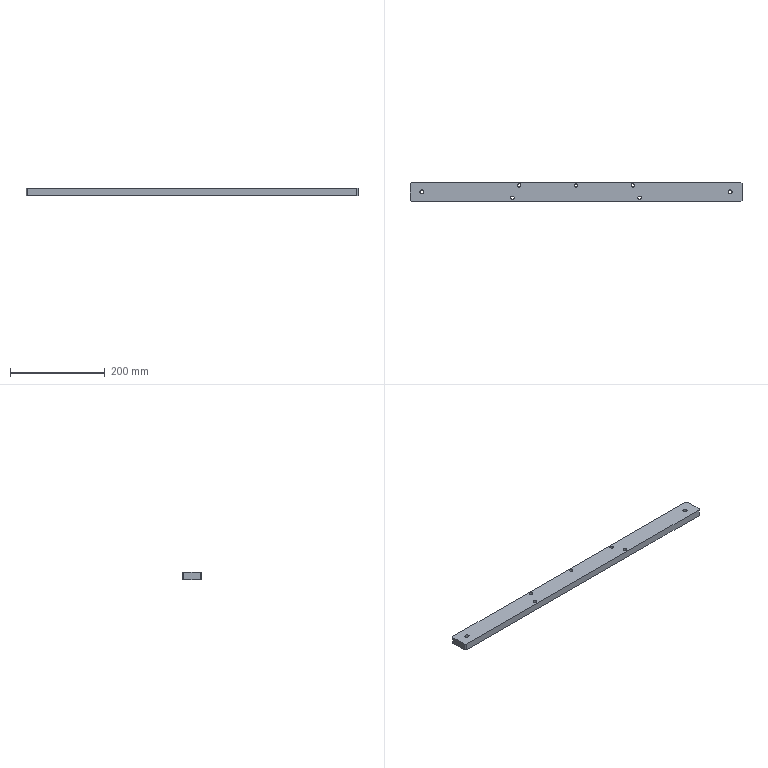Part | SolidWorks | features HoleWzd 2, Chamfer 1, Extrusion 1 | 1 solid | 24 faces | box 700 x 40 x 15 mm | volume 415141 mm3 | cylinder 14 | plane 10 | commonest cylinder face diameters 7 x10 8.5 x4
STEP:
#1=CARTESIAN_POINT('',(466.5,-6.,0.));
#2=VERTEX_POINT('',#1);
#3=CARTESIAN_POINT('',(473.5,-6.,0.));
#4=VERTEX_POINT('',#3);
#5=CARTESIAN_POINT('',(470.,-6.,0.));
#6=DIRECTION('',(0.,0.,1.));
#7=DIRECTION('',(1.,0.,0.));
#8=AXIS2_PLACEMENT_3D('',#5,#6,#7);
#9=CIRCLE('',#8,3.5);
#10=EDGE_CURVE('',#2,#4,#9,.T.);
#11=ORIENTED_EDGE('',*,*,#10,.F.);
#12=CARTESIAN_POINT('',(466.5,-6.,15.));
#13=VERTEX_POINT('',#12);
#14=CARTESIAN_POINT('',(466.5,-6.,15.));
#15=DIRECTION('',(0.,0.,1.));
#16=VECTOR('',#15,1000.);
#17=LINE('',#14,#16);
#18=EDGE_CURVE('',#2,#13,#17,.T.);
#19=ORIENTED_EDGE('',*,*,#18,.T.);
#20=CARTESIAN_POINT('',(473.5,-6.,15.));
#21=VERTEX_POINT('',#20);
#22=CARTESIAN_POINT('',(470.,-6.,15.));
#23=DIRECTION('',(0.,0.,1.));
#24=DIRECTION('',(1.,0.,0.));
#25=AXIS2_PLACEMENT_3D('',#22,#23,#24);
#26=CIRCLE('',#25,3.5);
#27=EDGE_CURVE('',#13,#21,#26,.T.);
#28=ORIENTED_EDGE('',*,*,#27,.T.);
#29=CARTESIAN_POINT('',(473.5,-6.,15.));
#30=DIRECTION('',(0.,0.,1.));
#31=VECTOR('',#30,1000.);
#32=LINE('',#29,#31);
#33=EDGE_CURVE('',#4,#21,#32,.T.);
#34=ORIENTED_EDGE('',*,*,#33,.F.);
#35=EDGE_LOOP('',(#11,#19,#28,#34));
#36=FACE_OUTER_BOUND('',#35,.T.);
#37=CARTESIAN_POINT('',(470.,-6.,15.));
#38=DIRECTION('',(0.,0.,1.));
#39=DIRECTION('',(1.,0.,0.));
#40=AXIS2_PLACEMENT_3D('',#37,#38,#39);
#41=CYLINDRICAL_SURFACE('',#40,3.5);
#42=ADVANCED_FACE('',(#36),#41,.F.);
#43=CARTESIAN_POINT('',(346.5,-6.,0.));
#44=VERTEX_POINT('',#43);
#45=CARTESIAN_POINT('',(353.5,-6.,0.));
#46=VERTEX_POINT('',#45);
#47=CARTESIAN_POINT('',(350.,-6.,0.));
#48=DIRECTION('',(0.,0.,1.));
#49=DIRECTION('',(1.,0.,0.));
#50=AXIS2_PLACEMENT_3D('',#47,#48,#49);
#51=CIRCLE('',#50,3.5);
#52=EDGE_CURVE('',#44,#46,#51,.T.);
#53=ORIENTED_EDGE('',*,*,#52,.F.);
#54=CARTESIAN_POINT('',(346.5,-6.,15.));
#55=VERTEX_POINT('',#54);
#56=CARTESIAN_POINT('',(346.5,-6.,15.));
#57=DIRECTION('',(0.,0.,1.));
#58=VECTOR('',#57,1000.);
#59=LINE('',#56,#58);
#60=EDGE_CURVE('',#44,#55,#59,.T.);
#61=ORIENTED_EDGE('',*,*,#60,.T.);
#62=CARTESIAN_POINT('',(353.5,-6.,15.));
#63=VERTEX_POINT('',#62);
#64=CARTESIAN_POINT('',(350.,-6.,15.));
#65=DIRECTION('',(0.,0.,1.));
#66=DIRECTION('',(1.,0.,0.));
#67=AXIS2_PLACEMENT_3D('',#64,#65,#66);
#68=CIRCLE('',#67,3.5);
#69=EDGE_CURVE('',#55,#63,#68,.T.);
#70=ORIENTED_EDGE('',*,*,#69,.T.);
#71=CARTESIAN_POINT('',(353.5,-6.,15.));
#72=DIRECTION('',(0.,0.,1.));
#73=VECTOR('',#72,1000.);
#74=LINE('',#71,#73);
#75=EDGE_CURVE('',#46,#63,#74,.T.);
#76=ORIENTED_EDGE('',*,*,#75,.F.);
#77=EDGE_LOOP('',(#53,#61,#70,#76));
#78=FACE_OUTER_BOUND('',#77,.T.);
#79=CARTESIAN_POINT('',(350.,-6.,15.));
#80=DIRECTION('',(0.,0.,1.));
#81=DIRECTION('',(1.,0.,0.));
#82=AXIS2_PLACEMENT_3D('',#79,#80,#81);
#83=CYLINDRICAL_SURFACE('',#82,3.5);
#84=ADVANCED_FACE('',(#78),#83,.F.);
#85=CARTESIAN_POINT('',(226.5,-6.,0.));
#86=VERTEX_POINT('',#85);
#87=CARTESIAN_POINT('',(233.5,-6.,0.));
#88=VERTEX_POINT('',#87);
#89=CARTESIAN_POINT('',(230.,-6.,0.));
#90=DIRECTION('',(0.,0.,1.));
#91=DIRECTION('',(1.,0.,0.));
#92=AXIS2_PLACEMENT_3D('',#89,#90,#91);
#93=CIRCLE('',#92,3.5);
#94=EDGE_CURVE('',#86,#88,#93,.T.);
#95=ORIENTED_EDGE('',*,*,#94,.F.);
#96=CARTESIAN_POINT('',(226.5,-6.,15.));
#97=VERTEX_POINT('',#96);
#98=CARTESIAN_POINT('',(226.5,-6.,15.));
#99=DIRECTION('',(0.,0.,1.));
#100=VECTOR('',#99,1000.);
#101=LINE('',#98,#100);
#102=EDGE_CURVE('',#86,#97,#101,.T.);
#103=ORIENTED_EDGE('',*,*,#102,.T.);
#104=CARTESIAN_POINT('',(233.5,-6.,15.));
#105=VERTEX_POINT('',#104);
#106=CARTESIAN_POINT('',(230.,-6.,15.));
#107=DIRECTION('',(0.,0.,1.));
#108=DIRECTION('',(1.,0.,0.));
#109=AXIS2_PLACEMENT_3D('',#106,#107,#108);
#110=CIRCLE('',#109,3.5);
#111=EDGE_CURVE('',#97,#105,#110,.T.);
#112=ORIENTED_EDGE('',*,*,#111,.T.);
#113=CARTESIAN_POINT('',(233.5,-6.,15.));
#114=DIRECTION('',(0.,0.,1.));
#115=VECTOR('',#114,1000.);
#116=LINE('',#113,#115);
#117=EDGE_CURVE('',#88,#105,#116,.T.);
#118=ORIENTED_EDGE('',*,*,#117,.F.);
#119=EDGE_LOOP('',(#95,#103,#112,#118));
#120=FACE_OUTER_BOUND('',#119,.T.);
#121=CARTESIAN_POINT('',(230.,-6.,15.));
#122=DIRECTION('',(0.,0.,1.));
#123=DIRECTION('',(1.,0.,0.));
#124=AXIS2_PLACEMENT_3D('',#121,#122,#123);
#125=CYLINDRICAL_SURFACE('',#124,3.5);
#126=ADVANCED_FACE('',(#120),#125,.F.);
#127=CARTESIAN_POINT('',(212.5,-32.,0.));
#128=VERTEX_POINT('',#127);
#129=CARTESIAN_POINT('',(219.5,-32.,0.));
#130=VERTEX_POINT('',#129);
#131=CARTESIAN_POINT('',(216.,-32.,0.));
#132=DIRECTION('',(0.,0.,1.));
#133=DIRECTION('',(1.,0.,0.));
#134=AXIS2_PLACEMENT_3D('',#131,#132,#133);
#135=CIRCLE('',#134,3.5);
#136=EDGE_CURVE('',#128,#130,#135,.T.);
#137=ORIENTED_EDGE('',*,*,#136,.F.);
#138=CARTESIAN_POINT('',(212.5,-32.,15.));
#139=VERTEX_POINT('',#138);
#140=CARTESIAN_POINT('',(212.5,-32.,15.));
#141=DIRECTION('',(0.,0.,1.));
#142=VECTOR('',#141,1000.);
#143=LINE('',#140,#142);
#144=EDGE_CURVE('',#128,#139,#143,.T.);
#145=ORIENTED_EDGE('',*,*,#144,.T.);
#146=CARTESIAN_POINT('',(219.5,-32.,15.));
#147=VERTEX_POINT('',#146);
#148=CARTESIAN_POINT('',(216.,-32.,15.));
#149=DIRECTION('',(0.,0.,1.));
#150=DIRECTION('',(1.,0.,0.));
#151=AXIS2_PLACEMENT_3D('',#148,#149,#150);
#152=CIRCLE('',#151,3.5);
#153=EDGE_CURVE('',#139,#147,#152,.T.);
#154=ORIENTED_EDGE('',*,*,#153,.T.);
#155=CARTESIAN_POINT('',(219.5,-32.,15.));
#156=DIRECTION('',(0.,0.,1.));
#157=VECTOR('',#156,1000.);
#158=LINE('',#155,#157);
#159=EDGE_CURVE('',#130,#147,#158,.T.);
#160=ORIENTED_EDGE('',*,*,#159,.F.);
#161=EDGE_LOOP('',(#137,#145,#154,#160));
#162=FACE_OUTER_BOUND('',#161,.T.);
#163=CARTESIAN_POINT('',(216.,-32.,15.));
#164=DIRECTION('',(0.,0.,1.));
#165=DIRECTION('',(1.,0.,0.));
#166=AXIS2_PLACEMENT_3D('',#163,#164,#165);
#167=CYLINDRICAL_SURFACE('',#166,3.5);
#168=ADVANCED_FACE('',(#162),#167,.F.);
#169=CARTESIAN_POINT('',(480.5,-32.,0.));
#170=VERTEX_POINT('',#169);
#171=CARTESIAN_POINT('',(487.5,-32.,0.));
#172=VERTEX_POINT('',#171);
#173=CARTESIAN_POINT('',(484.,-32.,0.));
#174=DIRECTION('',(0.,0.,1.));
#175=DIRECTION('',(1.,0.,0.));
#176=AXIS2_PLACEMENT_3D('',#173,#174,#175);
#177=CIRCLE('',#176,3.5);
#178=EDGE_CURVE('',#170,#172,#177,.T.);
#179=ORIENTED_EDGE('',*,*,#178,.F.);
#180=CARTESIAN_POINT('',(480.5,-32.,15.));
#181=VERTEX_POINT('',#180);
#182=CARTESIAN_POINT('',(480.5,-32.,15.));
#183=DIRECTION('',(0.,0.,1.));
#184=VECTOR('',#183,1000.);
#185=LINE('',#182,#184);
#186=EDGE_CURVE('',#170,#181,#185,.T.);
#187=ORIENTED_EDGE('',*,*,#186,.T.);
#188=CARTESIAN_POINT('',(487.5,-32.,15.));
#189=VERTEX_POINT('',#188);
#190=CARTESIAN_POINT('',(484.,-32.,15.));
#191=DIRECTION('',(0.,0.,1.));
#192=DIRECTION('',(1.,0.,0.));
#193=AXIS2_PLACEMENT_3D('',#190,#191,#192);
#194=CIRCLE('',#193,3.5);
#195=EDGE_CURVE('',#181,#189,#194,.T.);
#196=ORIENTED_EDGE('',*,*,#195,.T.);
#197=CARTESIAN_POINT('',(487.5,-32.,15.));
#198=DIRECTION('',(0.,0.,1.));
#199=VECTOR('',#198,1000.);
#200=LINE('',#197,#199);
#201=EDGE_CURVE('',#172,#189,#200,.T.);
#202=ORIENTED_EDGE('',*,*,#201,.F.);
#203=EDGE_LOOP('',(#179,#187,#196,#202));
#204=FACE_OUTER_BOUND('',#203,.T.);
#205=CARTESIAN_POINT('',(484.,-32.,15.));
#206=DIRECTION('',(0.,0.,1.));
#207=DIRECTION('',(1.,0.,0.));
#208=AXIS2_PLACEMENT_3D('',#205,#206,#207);
#209=CYLINDRICAL_SURFACE('',#208,3.5);
#210=ADVANCED_FACE('',(#204),#209,.F.);
#211=CARTESIAN_POINT('',(20.75,-20.,0.));
#212=VERTEX_POINT('',#211);
#213=CARTESIAN_POINT('',(29.25,-20.,0.));
#214=VERTEX_POINT('',#213);
#215=CARTESIAN_POINT('',(25.,-20.,0.));
#216=DIRECTION('',(0.,0.,1.));
#217=DIRECTION('',(1.,0.,0.));
#218=AXIS2_PLACEMENT_3D('',#215,#216,#217);
#219=CIRCLE('',#218,4.25);
#220=EDGE_CURVE('',#212,#214,#219,.T.);
#221=ORIENTED_EDGE('',*,*,#220,.F.);
#222=CARTESIAN_POINT('',(20.75,-20.,15.));
#223=VERTEX_POINT('',#222);
#224=CARTESIAN_POINT('',(20.75,-20.,15.));
#225=DIRECTION('',(0.,0.,1.));
#226=VECTOR('',#225,1000.);
#227=LINE('',#224,#226);
#228=EDGE_CURVE('',#212,#223,#227,.T.);
#229=ORIENTED_EDGE('',*,*,#228,.T.);
#230=CARTESIAN_POINT('',(29.25,-20.,15.));
#231=VERTEX_POINT('',#230);
#232=CARTESIAN_POINT('',(25.,-20.,15.));
#233=DIRECTION('',(0.,0.,1.));
#234=DIRECTION('',(1.,0.,0.));
#235=AXIS2_PLACEMENT_3D('',#232,#233,#234);
#236=CIRCLE('',#235,4.25);
#237=EDGE_CURVE('',#223,#231,#236,.T.);
#238=ORIENTED_EDGE('',*,*,#237,.T.);
#239=CARTESIAN_POINT('',(29.25,-20.,15.));
#240=DIRECTION('',(0.,0.,1.));
#241=VECTOR('',#240,1000.);
#242=LINE('',#239,#241);
#243=EDGE_CURVE('',#214,#231,#242,.T.);
#244=ORIENTED_EDGE('',*,*,#243,.F.);
#245=EDGE_LOOP('',(#221,#229,#238,#244));
#246=FACE_OUTER_BOUND('',#245,.T.);
#247=CARTESIAN_POINT('',(25.,-20.,15.));
#248=DIRECTION('',(0.,0.,1.));
#249=DIRECTION('',(1.,0.,0.));
#250=AXIS2_PLACEMENT_3D('',#247,#248,#249);
#251=CYLINDRICAL_SURFACE('',#250,4.25);
#252=ADVANCED_FACE('',(#246),#251,.F.);
#253=CARTESIAN_POINT('',(670.75,-20.,0.));
#254=VERTEX_POINT('',#253);
#255=CARTESIAN_POINT('',(679.25,-20.,0.));
#256=VERTEX_POINT('',#255);
#257=CARTESIAN_POINT('',(675.,-20.,0.));
#258=DIRECTION('',(0.,0.,1.));
#259=DIRECTION('',(1.,0.,0.));
#260=AXIS2_PLACEMENT_3D('',#257,#258,#259);
#261=CIRCLE('',#260,4.25);
#262=EDGE_CURVE('',#254,#256,#261,.T.);
#263=ORIENTED_EDGE('',*,*,#262,.F.);
#264=CARTESIAN_POINT('',(670.75,-20.,15.));
#265=VERTEX_POINT('',#264);
#266=CARTESIAN_POINT('',(670.75,-20.,15.));
#267=DIRECTION('',(0.,0.,1.));
#268=VECTOR('',#267,1000.);
#269=LINE('',#266,#268);
#270=EDGE_CURVE('',#254,#265,#269,.T.);
#271=ORIENTED_EDGE('',*,*,#270,.T.);
#272=CARTESIAN_POINT('',(679.25,-20.,15.));
#273=VERTEX_POINT('',#272);
#274=CARTESIAN_POINT('',(675.,-20.,15.));
#275=DIRECTION('',(0.,0.,1.));
#276=DIRECTION('',(1.,0.,0.));
#277=AXIS2_PLACEMENT_3D('',#274,#275,#276);
#278=CIRCLE('',#277,4.25);
#279=EDGE_CURVE('',#265,#273,#278,.T.);
#280=ORIENTED_EDGE('',*,*,#279,.T.);
#281=CARTESIAN_POINT('',(679.25,-20.,15.));
#282=DIRECTION('',(0.,0.,1.));
#283=VECTOR('',#282,1000.);
#284=LINE('',#281,#283);
#285=EDGE_CURVE('',#256,#273,#284,.T.);
#286=ORIENTED_EDGE('',*,*,#285,.F.);
#287=EDGE_LOOP('',(#263,#271,#280,#286));
#288=FACE_OUTER_BOUND('',#287,.T.);
#289=CARTESIAN_POINT('',(675.,-20.,15.));
#290=DIRECTION('',(0.,0.,1.));
#291=DIRECTION('',(1.,0.,0.));
#292=AXIS2_PLACEMENT_3D('',#289,#290,#291);
#293=CYLINDRICAL_SURFACE('',#292,4.25);
#294=ADVANCED_FACE('',(#288),#293,.F.);
#295=CARTESIAN_POINT('',(0.,-3.,0.));
#296=VERTEX_POINT('',#295);
#297=CARTESIAN_POINT('',(0.,-37.,0.));
#298=VERTEX_POINT('',#297);
#299=CARTESIAN_POINT('',(0.,0.,0.));
#300=DIRECTION('',(0.,-1.,0.));
#301=VECTOR('',#300,1000.);
#302=LINE('',#299,#301);
#303=EDGE_CURVE('',#296,#298,#302,.T.);
#304=ORIENTED_EDGE('',*,*,#303,.T.);
#305=CARTESIAN_POINT('',(0.,-37.,15.));
#306=VERTEX_POINT('',#305);
#307=CARTESIAN_POINT('',(0.,-37.,15.));
#308=DIRECTION('',(0.,0.,1.));
#309=VECTOR('',#308,1000.);
#310=LINE('',#307,#309);
#311=EDGE_CURVE('',#298,#306,#310,.T.);
#312=ORIENTED_EDGE('',*,*,#311,.T.);
#313=CARTESIAN_POINT('',(0.,-3.,15.));
#314=VERTEX_POINT('',#313);
#315=CARTESIAN_POINT('',(0.,0.,15.));
#316=DIRECTION('',(0.,-1.,0.));
#317=VECTOR('',#316,1000.);
#318=LINE('',#315,#317);
#319=EDGE_CURVE('',#314,#306,#318,.T.);
#320=ORIENTED_EDGE('',*,*,#319,.F.);
#321=CARTESIAN_POINT('',(0.,-3.,15.));
#322=DIRECTION('',(0.,0.,-1.));
#323=VECTOR('',#322,1000.);
#324=LINE('',#321,#323);
#325=EDGE_CURVE('',#314,#296,#324,.T.);
#326=ORIENTED_EDGE('',*,*,#325,.T.);
#327=EDGE_LOOP('',(#304,#312,#320,#326));
#328=FACE_OUTER_BOUND('',#327,.T.);
#329=CARTESIAN_POINT('',(0.,0.,15.));
#330=DIRECTION('',(1.,0.,0.));
#331=DIRECTION('',(0.,1.,0.));
#332=AXIS2_PLACEMENT_3D('',#329,#330,#331);
#333=PLANE('',#332);
#334=ADVANCED_FACE('',(#328),#333,.F.);
#335=CARTESIAN_POINT('',(3.,-40.,0.));
#336=VERTEX_POINT('',#335);
#337=CARTESIAN_POINT('',(697.,-40.,0.));
#338=VERTEX_POINT('',#337);
#339=CARTESIAN_POINT('',(0.,-40.,0.));
#340=DIRECTION('',(1.,0.,0.));
#341=VECTOR('',#340,1000.);
#342=LINE('',#339,#341);
#343=EDGE_CURVE('',#336,#338,#342,.T.);
#344=ORIENTED_EDGE('',*,*,#343,.T.);
#345=CARTESIAN_POINT('',(697.,-40.,15.));
#346=VERTEX_POINT('',#345);
#347=CARTESIAN_POINT('',(697.,-40.,15.));
#348=DIRECTION('',(0.,0.,1.));
#349=VECTOR('',#348,1000.);
#350=LINE('',#347,#349);
#351=EDGE_CURVE('',#338,#346,#350,.T.);
#352=ORIENTED_EDGE('',*,*,#351,.T.);
#353=CARTESIAN_POINT('',(3.,-40.,15.));
#354=VERTEX_POINT('',#353);
#355=CARTESIAN_POINT('',(0.,-40.,15.));
#356=DIRECTION('',(1.,0.,0.));
#357=VECTOR('',#356,1000.);
#358=LINE('',#355,#357);
#359=EDGE_CURVE('',#354,#346,#358,.T.);
#360=ORIENTED_EDGE('',*,*,#359,.F.);
#361=CARTESIAN_POINT('',(3.,-40.,15.));
#362=DIRECTION('',(0.,0.,-1.));
#363=VECTOR('',#362,1000.);
#364=LINE('',#361,#363);
#365=EDGE_CURVE('',#354,#336,#364,.T.);
#366=ORIENTED_EDGE('',*,*,#365,.T.);
#367=EDGE_LOOP('',(#344,#352,#360,#366));
#368=FACE_OUTER_BOUND('',#367,.T.);
#369=CARTESIAN_POINT('',(0.,-40.,15.));
#370=DIRECTION('',(0.,1.,0.));
#371=DIRECTION('',(0.,0.,1.));
#372=AXIS2_PLACEMENT_3D('',#369,#370,#371);
#373=PLANE('',#372);
#374=ADVANCED_FACE('',(#368),#373,.F.);
#375=CARTESIAN_POINT('',(700.,-37.,15.));
#376=VERTEX_POINT('',#375);
#377=CARTESIAN_POINT('',(700.,-3.,15.));
#378=VERTEX_POINT('',#377);
#379=CARTESIAN_POINT('',(700.,0.,15.));
#380=DIRECTION('',(0.,1.,0.));
#381=VECTOR('',#380,1000.);
#382=LINE('',#379,#381);
#383=EDGE_CURVE('',#376,#378,#382,.T.);
#384=ORIENTED_EDGE('',*,*,#383,.F.);
#385=CARTESIAN_POINT('',(700.,-37.,0.));
#386=VERTEX_POINT('',#385);
#387=CARTESIAN_POINT('',(700.,-37.,15.));
#388=DIRECTION('',(0.,0.,-1.));
#389=VECTOR('',#388,1000.);
#390=LINE('',#387,#389);
#391=EDGE_CURVE('',#376,#386,#390,.T.);
#392=ORIENTED_EDGE('',*,*,#391,.T.);
#393=CARTESIAN_POINT('',(700.,-3.,0.));
#394=VERTEX_POINT('',#393);
#395=CARTESIAN_POINT('',(700.,0.,0.));
#396=DIRECTION('',(0.,1.,0.));
#397=VECTOR('',#396,1000.);
#398=LINE('',#395,#397);
#399=EDGE_CURVE('',#386,#394,#398,.T.);
#400=ORIENTED_EDGE('',*,*,#399,.T.);
#401=CARTESIAN_POINT('',(700.,-3.,15.));
#402=DIRECTION('',(0.,0.,1.));
#403=VECTOR('',#402,1000.);
#404=LINE('',#401,#403);
#405=EDGE_CURVE('',#394,#378,#404,.T.);
#406=ORIENTED_EDGE('',*,*,#405,.T.);
#407=EDGE_LOOP('',(#384,#392,#400,#406));
#408=FACE_OUTER_BOUND('',#407,.T.);
#409=CARTESIAN_POINT('',(700.,0.,15.));
#410=DIRECTION('',(-1.,0.,0.));
#411=DIRECTION('',(0.,0.,1.));
#412=AXIS2_PLACEMENT_3D('',#409,#410,#411);
#413=PLANE('',#412);
#414=ADVANCED_FACE('',(#408),#413,.F.);
#415=CARTESIAN_POINT('',(697.,0.,15.));
#416=VERTEX_POINT('',#415);
#417=CARTESIAN_POINT('',(3.,0.,15.));
#418=VERTEX_POINT('',#417);
#419=CARTESIAN_POINT('',(0.,0.,15.));
#420=DIRECTION('',(-1.,0.,0.));
#421=VECTOR('',#420,1000.);
#422=LINE('',#419,#421);
#423=EDGE_CURVE('',#416,#418,#422,.T.);
#424=ORIENTED_EDGE('',*,*,#423,.F.);
#425=CARTESIAN_POINT('',(697.,0.,0.));
#426=VERTEX_POINT('',#425);
#427=CARTESIAN_POINT('',(697.,0.,15.));
#428=DIRECTION('',(0.,0.,-1.));
#429=VECTOR('',#428,1000.);
#430=LINE('',#427,#429);
#431=EDGE_CURVE('',#416,#426,#430,.T.);
#432=ORIENTED_EDGE('',*,*,#431,.T.);
#433=CARTESIAN_POINT('',(3.,0.,0.));
#434=VERTEX_POINT('',#433);
#435=CARTESIAN_POINT('',(0.,0.,0.));
#436=DIRECTION('',(-1.,0.,0.));
#437=VECTOR('',#436,1000.);
#438=LINE('',#435,#437);
#439=EDGE_CURVE('',#426,#434,#438,.T.);
#440=ORIENTED_EDGE('',*,*,#439,.T.);
#441=CARTESIAN_POINT('',(3.,0.,15.));
#442=DIRECTION('',(0.,0.,1.));
#443=VECTOR('',#442,1000.);
#444=LINE('',#441,#443);
#445=EDGE_CURVE('',#434,#418,#444,.T.);
#446=ORIENTED_EDGE('',*,*,#445,.T.);
#447=EDGE_LOOP('',(#424,#432,#440,#446));
#448=FACE_OUTER_BOUND('',#447,.T.);
#449=CARTESIAN_POINT('',(0.,0.,15.));
#450=DIRECTION('',(0.,-1.,0.));
#451=DIRECTION('',(0.,0.,-1.));
#452=AXIS2_PLACEMENT_3D('',#449,#450,#451);
#453=PLANE('',#452);
#454=ADVANCED_FACE('',(#448),#453,.F.);
#455=CARTESIAN_POINT('',(470.,-6.,15.));
#456=DIRECTION('',(0.,0.,1.));
#457=DIRECTION('',(1.,0.,0.));
#458=AXIS2_PLACEMENT_3D('',#455,#456,#457);
#459=CIRCLE('',#458,3.5);
#460=EDGE_CURVE('',#21,#13,#459,.T.);
#461=ORIENTED_EDGE('',*,*,#460,.F.);
#462=ORIENTED_EDGE('',*,*,#27,.F.);
#463=EDGE_LOOP('',(#461,#462));
#464=FACE_BOUND('',#463,.T.);
#465=CARTESIAN_POINT('',(350.,-6.,15.));
#466=DIRECTION('',(0.,0.,1.));
#467=DIRECTION('',(1.,0.,0.));
#468=AXIS2_PLACEMENT_3D('',#465,#466,#467);
#469=CIRCLE('',#468,3.5);
#470=EDGE_CURVE('',#63,#55,#469,.T.);
#471=ORIENTED_EDGE('',*,*,#470,.F.);
#472=ORIENTED_EDGE('',*,*,#69,.F.);
#473=EDGE_LOOP('',(#471,#472));
#474=FACE_BOUND('',#473,.T.);
#475=CARTESIAN_POINT('',(230.,-6.,15.));
#476=DIRECTION('',(0.,0.,1.));
#477=DIRECTION('',(1.,0.,0.));
#478=AXIS2_PLACEMENT_3D('',#475,#476,#477);
#479=CIRCLE('',#478,3.5);
#480=EDGE_CURVE('',#105,#97,#479,.T.);
#481=ORIENTED_EDGE('',*,*,#480,.F.);
#482=ORIENTED_EDGE('',*,*,#111,.F.);
#483=EDGE_LOOP('',(#481,#482));
#484=FACE_BOUND('',#483,.T.);
#485=CARTESIAN_POINT('',(216.,-32.,15.));
#486=DIRECTION('',(0.,0.,1.));
#487=DIRECTION('',(1.,0.,0.));
#488=AXIS2_PLACEMENT_3D('',#485,#486,#487);
#489=CIRCLE('',#488,3.5);
#490=EDGE_CURVE('',#147,#139,#489,.T.);
#491=ORIENTED_EDGE('',*,*,#490,.F.);
#492=ORIENTED_EDGE('',*,*,#153,.F.);
#493=EDGE_LOOP('',(#491,#492));
#494=FACE_BOUND('',#493,.T.);
#495=CARTESIAN_POINT('',(484.,-32.,15.));
#496=DIRECTION('',(0.,0.,1.));
#497=DIRECTION('',(1.,0.,0.));
#498=AXIS2_PLACEMENT_3D('',#495,#496,#497);
#499=CIRCLE('',#498,3.5);
#500=EDGE_CURVE('',#189,#181,#499,.T.);
#501=ORIENTED_EDGE('',*,*,#500,.F.);
#502=ORIENTED_EDGE('',*,*,#195,.F.);
#503=EDGE_LOOP('',(#501,#502));
#504=FACE_BOUND('',#503,.T.);
#505=CARTESIAN_POINT('',(25.,-20.,15.));
#506=DIRECTION('',(0.,0.,1.));
#507=DIRECTION('',(1.,0.,0.));
#508=AXIS2_PLACEMENT_3D('',#505,#506,#507);
#509=CIRCLE('',#508,4.25);
#510=EDGE_CURVE('',#231,#223,#509,.T.);
#511=ORIENTED_EDGE('',*,*,#510,.F.);
#512=ORIENTED_EDGE('',*,*,#237,.F.);
#513=EDGE_LOOP('',(#511,#512));
#514=FACE_BOUND('',#513,.T.);
#515=CARTESIAN_POINT('',(675.,-20.,15.));
#516=DIRECTION('',(0.,0.,1.));
#517=DIRECTION('',(1.,0.,0.));
#518=AXIS2_PLACEMENT_3D('',#515,#516,#517);
#519=CIRCLE('',#518,4.25);
#520=EDGE_CURVE('',#273,#265,#519,.T.);
#521=ORIENTED_EDGE('',*,*,#520,.F.);
#522=ORIENTED_EDGE('',*,*,#279,.F.);
#523=EDGE_LOOP('',(#521,#522));
#524=FACE_BOUND('',#523,.T.);
#525=ORIENTED_EDGE('',*,*,#359,.T.);
#526=CARTESIAN_POINT('',(368.5,-368.5,15.));
#527=DIRECTION('',(0.7071,0.7071,0.));
#528=VECTOR('',#527,1000.);
#529=LINE('',#526,#528);
#530=EDGE_CURVE('',#346,#376,#529,.T.);
#531=ORIENTED_EDGE('',*,*,#530,.T.);
#532=ORIENTED_EDGE('',*,*,#383,.T.);
#533=CARTESIAN_POINT('',(348.5,348.5,15.));
#534=DIRECTION('',(-0.7071,0.7071,0.));
#535=VECTOR('',#534,1000.);
#536=LINE('',#533,#535);
#537=EDGE_CURVE('',#378,#416,#536,.T.);
#538=ORIENTED_EDGE('',*,*,#537,.T.);
#539=ORIENTED_EDGE('',*,*,#423,.T.);
#540=CARTESIAN_POINT('',(1.5,-1.5,15.));
#541=DIRECTION('',(-0.7071,-0.7071,0.));
#542=VECTOR('',#541,1000.);
#543=LINE('',#540,#542);
#544=EDGE_CURVE('',#418,#314,#543,.T.);
#545=ORIENTED_EDGE('',*,*,#544,.T.);
#546=ORIENTED_EDGE('',*,*,#319,.T.);
#547=CARTESIAN_POINT('',(-18.5,-18.5,15.));
#548=DIRECTION('',(0.7071,-0.7071,0.));
#549=VECTOR('',#548,1000.);
#550=LINE('',#547,#549);
#551=EDGE_CURVE('',#306,#354,#550,.T.);
#552=ORIENTED_EDGE('',*,*,#551,.T.);
#553=EDGE_LOOP('',(#525,#531,#532,#538,#539,#545,#546,#552));
#554=FACE_OUTER_BOUND('',#553,.T.);
#555=CARTESIAN_POINT('',(0.,0.,15.));
#556=DIRECTION('',(0.,0.,1.));
#557=DIRECTION('',(1.,0.,0.));
#558=AXIS2_PLACEMENT_3D('',#555,#556,#557);
#559=PLANE('',#558);
#560=ADVANCED_FACE('',(#464,#474,#484,#494,#504,#514,#524,#554),#559,.T.);
#561=CARTESIAN_POINT('',(470.,-6.,0.));
#562=DIRECTION('',(0.,0.,1.));
#563=DIRECTION('',(1.,0.,0.));
#564=AXIS2_PLACEMENT_3D('',#561,#562,#563);
#565=CIRCLE('',#564,3.5);
#566=EDGE_CURVE('',#4,#2,#565,.T.);
#567=ORIENTED_EDGE('',*,*,#566,.T.);
#568=ORIENTED_EDGE('',*,*,#10,.T.);
#569=EDGE_LOOP('',(#567,#568));
#570=FACE_BOUND('',#569,.T.);
#571=CARTESIAN_POINT('',(350.,-6.,0.));
#572=DIRECTION('',(0.,0.,1.));
#573=DIRECTION('',(1.,0.,0.));
#574=AXIS2_PLACEMENT_3D('',#571,#572,#573);
#575=CIRCLE('',#574,3.5);
#576=EDGE_CURVE('',#46,#44,#575,.T.);
#577=ORIENTED_EDGE('',*,*,#576,.T.);
#578=ORIENTED_EDGE('',*,*,#52,.T.);
#579=EDGE_LOOP('',(#577,#578));
#580=FACE_BOUND('',#579,.T.);
#581=CARTESIAN_POINT('',(230.,-6.,0.));
#582=DIRECTION('',(0.,0.,1.));
#583=DIRECTION('',(1.,0.,0.));
#584=AXIS2_PLACEMENT_3D('',#581,#582,#583);
#585=CIRCLE('',#584,3.5);
#586=EDGE_CURVE('',#88,#86,#585,.T.);
#587=ORIENTED_EDGE('',*,*,#586,.T.);
#588=ORIENTED_EDGE('',*,*,#94,.T.);
#589=EDGE_LOOP('',(#587,#588));
#590=FACE_BOUND('',#589,.T.);
#591=CARTESIAN_POINT('',(216.,-32.,0.));
#592=DIRECTION('',(0.,0.,1.));
#593=DIRECTION('',(1.,0.,0.));
#594=AXIS2_PLACEMENT_3D('',#591,#592,#593);
#595=CIRCLE('',#594,3.5);
#596=EDGE_CURVE('',#130,#128,#595,.T.);
#597=ORIENTED_EDGE('',*,*,#596,.T.);
#598=ORIENTED_EDGE('',*,*,#136,.T.);
#599=EDGE_LOOP('',(#597,#598));
#600=FACE_BOUND('',#599,.T.);
#601=CARTESIAN_POINT('',(484.,-32.,0.));
#602=DIRECTION('',(0.,0.,1.));
#603=DIRECTION('',(1.,0.,0.));
#604=AXIS2_PLACEMENT_3D('',#601,#602,#603);
#605=CIRCLE('',#604,3.5);
#606=EDGE_CURVE('',#172,#170,#605,.T.);
#607=ORIENTED_EDGE('',*,*,#606,.T.);
#608=ORIENTED_EDGE('',*,*,#178,.T.);
#609=EDGE_LOOP('',(#607,#608));
#610=FACE_BOUND('',#609,.T.);
#611=CARTESIAN_POINT('',(25.,-20.,0.));
#612=DIRECTION('',(0.,0.,1.));
#613=DIRECTION('',(1.,0.,0.));
#614=AXIS2_PLACEMENT_3D('',#611,#612,#613);
#615=CIRCLE('',#614,4.25);
#616=EDGE_CURVE('',#214,#212,#615,.T.);
#617=ORIENTED_EDGE('',*,*,#616,.T.);
#618=ORIENTED_EDGE('',*,*,#220,.T.);
#619=EDGE_LOOP('',(#617,#618));
#620=FACE_BOUND('',#619,.T.);
#621=CARTESIAN_POINT('',(675.,-20.,0.));
#622=DIRECTION('',(0.,0.,1.));
#623=DIRECTION('',(1.,0.,0.));
#624=AXIS2_PLACEMENT_3D('',#621,#622,#623);
#625=CIRCLE('',#624,4.25);
#626=EDGE_CURVE('',#256,#254,#625,.T.);
#627=ORIENTED_EDGE('',*,*,#626,.T.);
#628=ORIENTED_EDGE('',*,*,#262,.T.);
#629=EDGE_LOOP('',(#627,#628));
#630=FACE_BOUND('',#629,.T.);
#631=ORIENTED_EDGE('',*,*,#399,.F.);
#632=CARTESIAN_POINT('',(700.,-37.,0.));
#633=DIRECTION('',(-0.7071,-0.7071,0.));
#634=VECTOR('',#633,1000.);
#635=LINE('',#632,#634);
#636=EDGE_CURVE('',#386,#338,#635,.T.);
#637=ORIENTED_EDGE('',*,*,#636,.T.);
#638=ORIENTED_EDGE('',*,*,#343,.F.);
#639=CARTESIAN_POINT('',(3.,-40.,0.));
#640=DIRECTION('',(-0.7071,0.7071,0.));
#641=VECTOR('',#640,1000.);
#642=LINE('',#639,#641);
#643=EDGE_CURVE('',#336,#298,#642,.T.);
#644=ORIENTED_EDGE('',*,*,#643,.T.);
#645=ORIENTED_EDGE('',*,*,#303,.F.);
#646=CARTESIAN_POINT('',(0.,-3.,0.));
#647=DIRECTION('',(0.7071,0.7071,0.));
#648=VECTOR('',#647,1000.);
#649=LINE('',#646,#648);
#650=EDGE_CURVE('',#296,#434,#649,.T.);
#651=ORIENTED_EDGE('',*,*,#650,.T.);
#652=ORIENTED_EDGE('',*,*,#439,.F.);
#653=CARTESIAN_POINT('',(697.,0.,0.));
#654=DIRECTION('',(0.7071,-0.7071,0.));
#655=VECTOR('',#654,1000.);
#656=LINE('',#653,#655);
#657=EDGE_CURVE('',#426,#394,#656,.T.);
#658=ORIENTED_EDGE('',*,*,#657,.T.);
#659=EDGE_LOOP('',(#631,#637,#638,#644,#645,#651,#652,#658));
#660=FACE_OUTER_BOUND('',#659,.T.);
#661=CARTESIAN_POINT('',(0.,0.,0.));
#662=DIRECTION('',(0.,0.,1.));
#663=DIRECTION('',(1.,0.,0.));
#664=AXIS2_PLACEMENT_3D('',#661,#662,#663);
#665=PLANE('',#664);
#666=ADVANCED_FACE('',(#570,#580,#590,#600,#610,#620,#630,#660),#665,.F.);
#667=ORIENTED_EDGE('',*,*,#530,.F.);
#668=ORIENTED_EDGE('',*,*,#351,.F.);
#669=ORIENTED_EDGE('',*,*,#636,.F.);
#670=ORIENTED_EDGE('',*,*,#391,.F.);
#671=EDGE_LOOP('',(#667,#668,#669,#670));
#672=FACE_OUTER_BOUND('',#671,.T.);
#673=CARTESIAN_POINT('',(700.,-37.,15.));
#674=DIRECTION('',(-0.7071,0.7071,0.));
#675=DIRECTION('',(0.,0.,-1.));
#676=AXIS2_PLACEMENT_3D('',#673,#674,#675);
#677=PLANE('',#676);
#678=ADVANCED_FACE('',(#672),#677,.F.);
#679=ORIENTED_EDGE('',*,*,#537,.F.);
#680=ORIENTED_EDGE('',*,*,#405,.F.);
#681=ORIENTED_EDGE('',*,*,#657,.F.);
#682=ORIENTED_EDGE('',*,*,#431,.F.);
#683=EDGE_LOOP('',(#679,#680,#681,#682));
#684=FACE_OUTER_BOUND('',#683,.T.);
#685=CARTESIAN_POINT('',(697.,0.,15.));
#686=DIRECTION('',(-0.7071,-0.7071,0.));
#687=DIRECTION('',(0.,0.,-1.));
#688=AXIS2_PLACEMENT_3D('',#685,#686,#687);
#689=PLANE('',#688);
#690=ADVANCED_FACE('',(#684),#689,.F.);
#691=ORIENTED_EDGE('',*,*,#551,.F.);
#692=ORIENTED_EDGE('',*,*,#311,.F.);
#693=ORIENTED_EDGE('',*,*,#643,.F.);
#694=ORIENTED_EDGE('',*,*,#365,.F.);
#695=EDGE_LOOP('',(#691,#692,#693,#694));
#696=FACE_OUTER_BOUND('',#695,.T.);
#697=CARTESIAN_POINT('',(3.,-40.,15.));
#698=DIRECTION('',(0.7071,0.7071,0.));
#699=DIRECTION('',(0.,0.,-1.));
#700=AXIS2_PLACEMENT_3D('',#697,#698,#699);
#701=PLANE('',#700);
#702=ADVANCED_FACE('',(#696),#701,.F.);
#703=ORIENTED_EDGE('',*,*,#544,.F.);
#704=ORIENTED_EDGE('',*,*,#445,.F.);
#705=ORIENTED_EDGE('',*,*,#650,.F.);
#706=ORIENTED_EDGE('',*,*,#325,.F.);
#707=EDGE_LOOP('',(#703,#704,#705,#706));
#708=FACE_OUTER_BOUND('',#707,.T.);
#709=CARTESIAN_POINT('',(0.,-3.,15.));
#710=DIRECTION('',(0.7071,-0.7071,0.));
#711=DIRECTION('',(0.,0.,-1.));
#712=AXIS2_PLACEMENT_3D('',#709,#710,#711);
#713=PLANE('',#712);
#714=ADVANCED_FACE('',(#708),#713,.F.);
#715=ORIENTED_EDGE('',*,*,#270,.F.);
#716=ORIENTED_EDGE('',*,*,#626,.F.);
#717=ORIENTED_EDGE('',*,*,#285,.T.);
#718=ORIENTED_EDGE('',*,*,#520,.T.);
#719=EDGE_LOOP('',(#715,#716,#717,#718));
#720=FACE_OUTER_BOUND('',#719,.T.);
#721=CARTESIAN_POINT('',(675.,-20.,15.));
#722=DIRECTION('',(0.,0.,1.));
#723=DIRECTION('',(1.,0.,0.));
#724=AXIS2_PLACEMENT_3D('',#721,#722,#723);
#725=CYLINDRICAL_SURFACE('',#724,4.25);
#726=ADVANCED_FACE('',(#720),#725,.F.);
#727=ORIENTED_EDGE('',*,*,#228,.F.);
#728=ORIENTED_EDGE('',*,*,#616,.F.);
#729=ORIENTED_EDGE('',*,*,#243,.T.);
#730=ORIENTED_EDGE('',*,*,#510,.T.);
#731=EDGE_LOOP('',(#727,#728,#729,#730));
#732=FACE_OUTER_BOUND('',#731,.T.);
#733=CARTESIAN_POINT('',(25.,-20.,15.));
#734=DIRECTION('',(0.,0.,1.));
#735=DIRECTION('',(1.,0.,0.));
#736=AXIS2_PLACEMENT_3D('',#733,#734,#735);
#737=CYLINDRICAL_SURFACE('',#736,4.25);
#738=ADVANCED_FACE('',(#732),#737,.F.);
#739=ORIENTED_EDGE('',*,*,#186,.F.);
#740=ORIENTED_EDGE('',*,*,#606,.F.);
#741=ORIENTED_EDGE('',*,*,#201,.T.);
#742=ORIENTED_EDGE('',*,*,#500,.T.);
#743=EDGE_LOOP('',(#739,#740,#741,#742));
#744=FACE_OUTER_BOUND('',#743,.T.);
#745=CARTESIAN_POINT('',(484.,-32.,15.));
#746=DIRECTION('',(0.,0.,1.));
#747=DIRECTION('',(1.,0.,0.));
#748=AXIS2_PLACEMENT_3D('',#745,#746,#747);
#749=CYLINDRICAL_SURFACE('',#748,3.5);
#750=ADVANCED_FACE('',(#744),#749,.F.);
#751=ORIENTED_EDGE('',*,*,#144,.F.);
#752=ORIENTED_EDGE('',*,*,#596,.F.);
#753=ORIENTED_EDGE('',*,*,#159,.T.);
#754=ORIENTED_EDGE('',*,*,#490,.T.);
#755=EDGE_LOOP('',(#751,#752,#753,#754));
#756=FACE_OUTER_BOUND('',#755,.T.);
#757=CARTESIAN_POINT('',(216.,-32.,15.));
#758=DIRECTION('',(0.,0.,1.));
#759=DIRECTION('',(1.,0.,0.));
#760=AXIS2_PLACEMENT_3D('',#757,#758,#759);
#761=CYLINDRICAL_SURFACE('',#760,3.5);
#762=ADVANCED_FACE('',(#756),#761,.F.);
#763=ORIENTED_EDGE('',*,*,#102,.F.);
#764=ORIENTED_EDGE('',*,*,#586,.F.);
#765=ORIENTED_EDGE('',*,*,#117,.T.);
#766=ORIENTED_EDGE('',*,*,#480,.T.);
#767=EDGE_LOOP('',(#763,#764,#765,#766));
#768=FACE_OUTER_BOUND('',#767,.T.);
#769=CARTESIAN_POINT('',(230.,-6.,15.));
#770=DIRECTION('',(0.,0.,1.));
#771=DIRECTION('',(1.,0.,0.));
#772=AXIS2_PLACEMENT_3D('',#769,#770,#771);
#773=CYLINDRICAL_SURFACE('',#772,3.5);
#774=ADVANCED_FACE('',(#768),#773,.F.);
#775=ORIENTED_EDGE('',*,*,#60,.F.);
#776=ORIENTED_EDGE('',*,*,#576,.F.);
#777=ORIENTED_EDGE('',*,*,#75,.T.);
#778=ORIENTED_EDGE('',*,*,#470,.T.);
#779=EDGE_LOOP('',(#775,#776,#777,#778));
#780=FACE_OUTER_BOUND('',#779,.T.);
#781=CARTESIAN_POINT('',(350.,-6.,15.));
#782=DIRECTION('',(0.,0.,1.));
#783=DIRECTION('',(1.,0.,0.));
#784=AXIS2_PLACEMENT_3D('',#781,#782,#783);
#785=CYLINDRICAL_SURFACE('',#784,3.5);
#786=ADVANCED_FACE('',(#780),#785,.F.);
#787=ORIENTED_EDGE('',*,*,#18,.F.);
#788=ORIENTED_EDGE('',*,*,#566,.F.);
#789=ORIENTED_EDGE('',*,*,#33,.T.);
#790=ORIENTED_EDGE('',*,*,#460,.T.);
#791=EDGE_LOOP('',(#787,#788,#789,#790));
#792=FACE_OUTER_BOUND('',#791,.T.);
#793=CARTESIAN_POINT('',(470.,-6.,15.));
#794=DIRECTION('',(0.,0.,1.));
#795=DIRECTION('',(1.,0.,0.));
#796=AXIS2_PLACEMENT_3D('',#793,#794,#795);
#797=CYLINDRICAL_SURFACE('',#796,3.5);
#798=ADVANCED_FACE('',(#792),#797,.F.);
#799=CLOSED_SHELL('',(#42,#84,#126,#168,#210,#252,#294,#334,#374,#414,#454,#560,#666,#678,#690,#702,#714,#726,#738,#750,#762,#774,#786,#798));
#800=MANIFOLD_SOLID_BREP('',#799);
#801=CARTESIAN_POINT('',(0.,0.,0.));
#802=DIRECTION('',(0.,0.,1.));
#803=DIRECTION('',(1.,0.,0.));
#804=AXIS2_PLACEMENT_3D('',#801,#802,#803);
#805=(LENGTH_UNIT()NAMED_UNIT(*)SI_UNIT(.MILLI.,.METRE.));
#806=UNCERTAINTY_MEASURE_WITH_UNIT(LENGTH_MEASURE(0.00001),#805,'','');
#807=(NAMED_UNIT(*)PLANE_ANGLE_UNIT()SI_UNIT($,.RADIAN.));
#808=(NAMED_UNIT(*)SI_UNIT($,.STERADIAN.)SOLID_ANGLE_UNIT());
#809=(GEOMETRIC_REPRESENTATION_CONTEXT(3)GLOBAL_UNCERTAINTY_ASSIGNED_CONTEXT((#806))GLOBAL_UNIT_ASSIGNED_CONTEXT((#805,#807,#808))REPRESENTATION_CONTEXT('',''));
#810=ADVANCED_BREP_SHAPE_REPRESENTATION('',(#800,#804),#809);